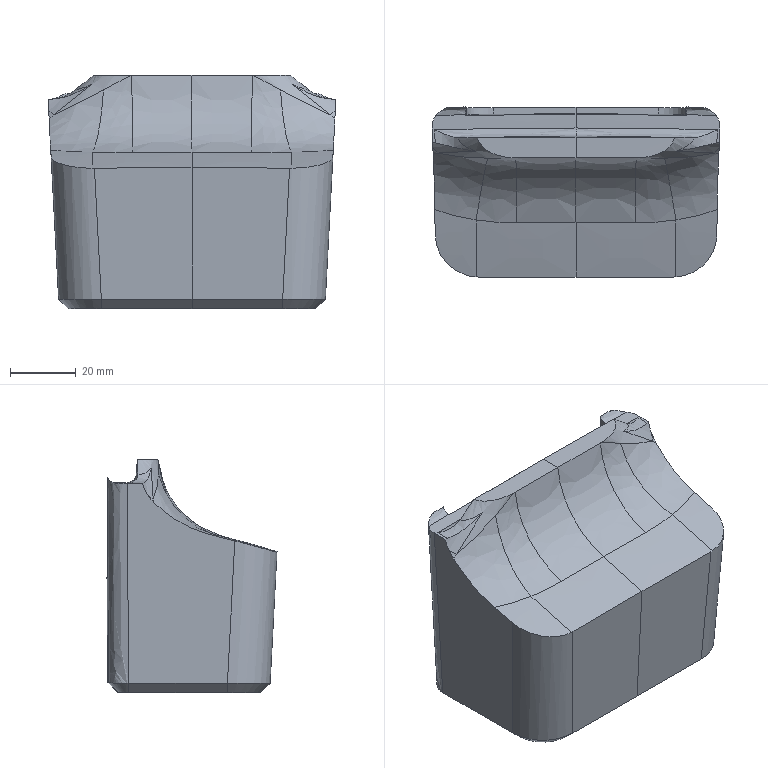Part | STEP file | solid 46 | 1 solid | 62 faces | volume 211233 mm3 | spline 47 | plane 7 | cylinder 6 | cone 2 | commonest cylinder face diameters 16.208 x2 26 x2 14 x1 25 x1